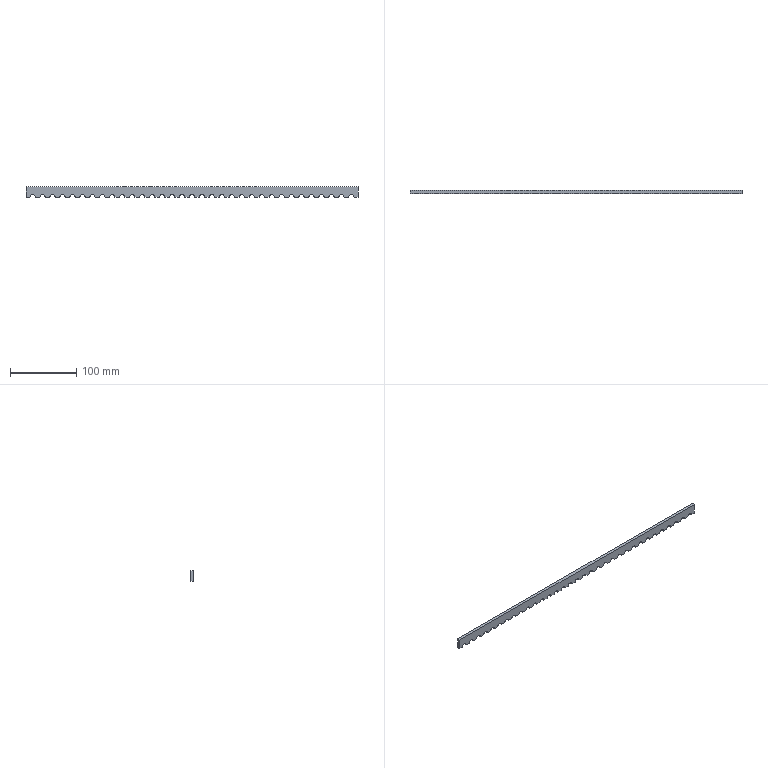Part | SolidWorks | features FlatPattern 1, ICE 1, SMBaseFlange 1, SheetMetal 1 | 1 solid | 105 faces | box 500 x 4.5 x 16 mm | volume 32268 mm3 | cylinder 66 | plane 39 | commonest cylinder face diameters 8 x66